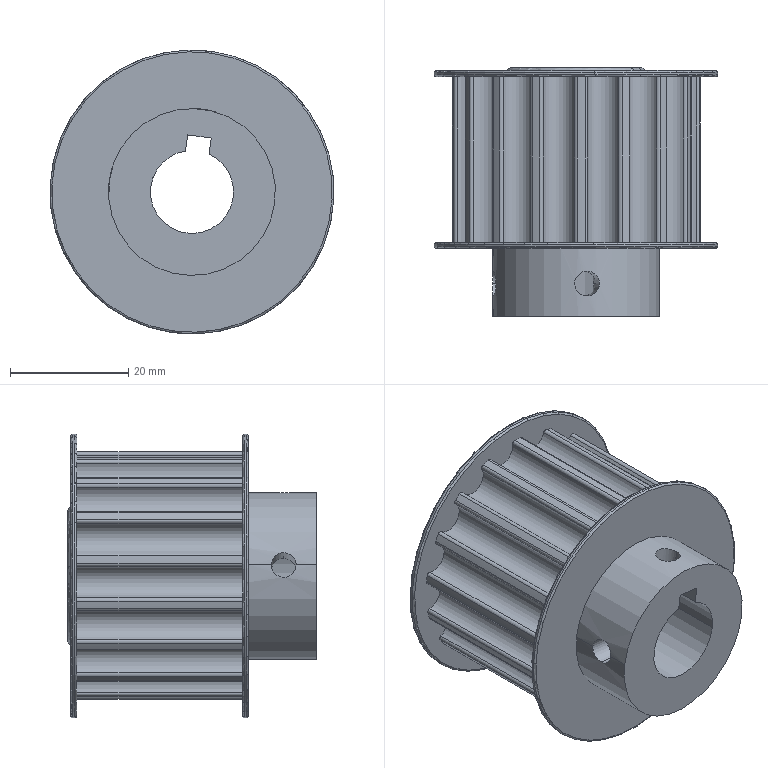Part | SolidWorks | features BaseBody 1 | 1 solid | 103 faces | box 48 x 42 x 48 mm | volume 35797 mm3 | cylinder 81 | plane 12 | torus 10 | commonest cylinder face diameters 1 x34 5.3 x17 41.98 x17 4.2 x4 48 x4 14.05 x3